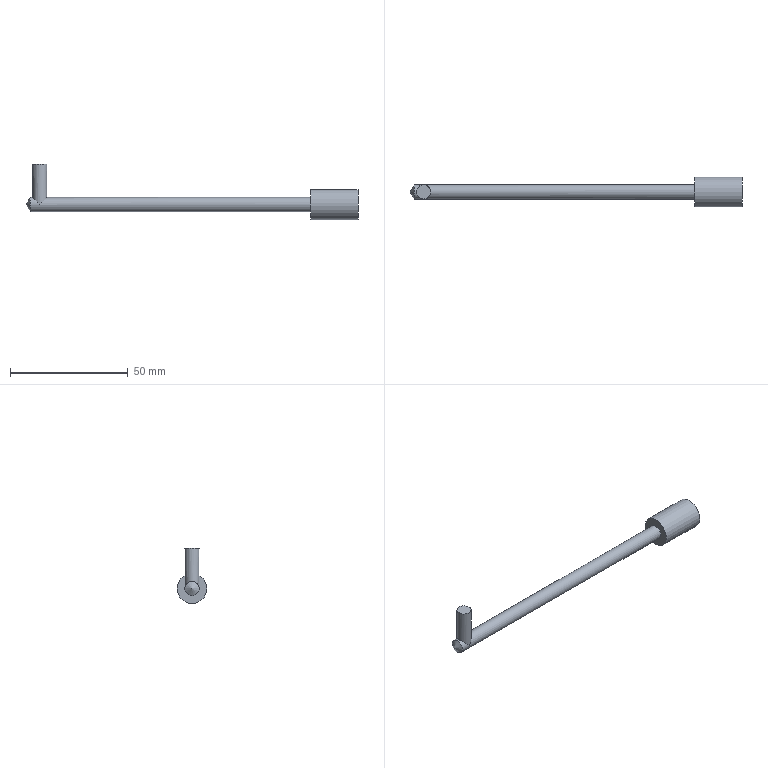Part | NX | features solid 2 | 1 solid | 7 faces | box 140.803 x 12.7 x 23.35 mm | volume 6324 mm3 | plane 3 | cylinder 3 | cone 1 | commonest cylinder face diameters 6 x2 12.7 x1
STEP:
#1=CARTESIAN_POINT('',(155.,30.,-84.));
#2=VERTEX_POINT('',#1);
#3=CARTESIAN_POINT('',(155.,30.,-87.));
#4=DIRECTION('',(-1.,0.,0.));
#5=DIRECTION('',(0.,0.,1.));
#6=AXIS2_PLACEMENT_3D('',#3,#4,#5);
#7=CIRCLE('',#6,3.);
#8=EDGE_CURVE('',#2,#2,#7,.T.);
#9=ORIENTED_EDGE('',*,*,#8,.F.);
#10=EDGE_LOOP('',(#9));
#11=FACE_BOUND('',#10,.T.);
#12=CARTESIAN_POINT('',(155.,30.,-80.65));
#13=VERTEX_POINT('',#12);
#14=CARTESIAN_POINT('',(155.,30.,-87.));
#15=DIRECTION('',(1.,0.,0.));
#16=DIRECTION('',(0.,0.,1.));
#17=AXIS2_PLACEMENT_3D('',#14,#15,#16);
#18=CIRCLE('',#17,6.35);
#19=EDGE_CURVE('',#13,#13,#18,.T.);
#20=ORIENTED_EDGE('',*,*,#19,.F.);
#21=EDGE_LOOP('',(#20));
#22=FACE_BOUND('',#21,.T.);
#23=CARTESIAN_POINT('',(155.,30.,-87.));
#24=DIRECTION('',(-1.,0.,0.));
#25=DIRECTION('',(0.,0.,1.));
#26=AXIS2_PLACEMENT_3D('',#23,#24,#25);
#27=PLANE('',#26);
#28=ADVANCED_FACE('',(#11,#22),#27,.T.);
#29=CARTESIAN_POINT('',(175.,30.,-80.65));
#30=VERTEX_POINT('',#29);
#31=CARTESIAN_POINT('',(175.,30.,-87.));
#32=DIRECTION('',(-1.,0.,0.));
#33=DIRECTION('',(0.,0.,1.));
#34=AXIS2_PLACEMENT_3D('',#31,#32,#33);
#35=CIRCLE('',#34,6.35);
#36=EDGE_CURVE('',#30,#30,#35,.T.);
#37=ORIENTED_EDGE('',*,*,#36,.F.);
#38=EDGE_LOOP('',(#37));
#39=FACE_BOUND('',#38,.T.);
#40=CARTESIAN_POINT('',(175.,30.,-87.));
#41=DIRECTION('',(1.,0.,0.));
#42=DIRECTION('',(0.,0.,-1.));
#43=AXIS2_PLACEMENT_3D('',#40,#41,#42);
#44=PLANE('',#43);
#45=ADVANCED_FACE('',(#39),#44,.T.);
#46=ORIENTED_EDGE('',*,*,#19,.T.);
#47=EDGE_LOOP('',(#46));
#48=FACE_BOUND('',#47,.T.);
#49=ORIENTED_EDGE('',*,*,#36,.T.);
#50=EDGE_LOOP('',(#49));
#51=FACE_BOUND('',#50,.T.);
#52=CARTESIAN_POINT('',(175.,30.,-87.));
#53=DIRECTION('',(-1.,0.,0.));
#54=DIRECTION('',(0.,0.,1.));
#55=AXIS2_PLACEMENT_3D('',#52,#53,#54);
#56=CYLINDRICAL_SURFACE('',#55,6.35);
#57=ADVANCED_FACE('',(#48,#51),#56,.T.);
#58=CARTESIAN_POINT('',(40.,33.,-87.));
#59=VERTEX_POINT('',#58);
#60=CARTESIAN_POINT('',(40.,27.,-87.));
#61=VERTEX_POINT('',#60);
#62=CARTESIAN_POINT('',(40.,30.,-87.));
#63=DIRECTION('',(-0.7071,0.,-0.7071));
#64=DIRECTION('',(-0.7071,0.,0.7071));
#65=AXIS2_PLACEMENT_3D('',#62,#63,#64);
#66=ELLIPSE('',#65,4.243,3.);
#67=EDGE_CURVE('',#59,#61,#66,.F.);
#68=ORIENTED_EDGE('',*,*,#67,.F.);
#69=CARTESIAN_POINT('',(40.,30.,-87.));
#70=DIRECTION('',(-0.7071,0.,0.7071));
#71=DIRECTION('',(-0.7071,0.,-0.7071));
#72=AXIS2_PLACEMENT_3D('',#69,#70,#71);
#73=ELLIPSE('',#72,4.243,3.);
#74=EDGE_CURVE('',#61,#59,#73,.T.);
#75=ORIENTED_EDGE('',*,*,#74,.F.);
#76=EDGE_LOOP('',(#68,#75));
#77=FACE_BOUND('',#76,.T.);
#78=ORIENTED_EDGE('',*,*,#8,.T.);
#79=EDGE_LOOP('',(#78));
#80=FACE_BOUND('',#79,.T.);
#81=CARTESIAN_POINT('',(36.,30.,-84.));
#82=VERTEX_POINT('',#81);
#83=CARTESIAN_POINT('',(36.,30.,-87.));
#84=DIRECTION('',(-1.,0.,0.));
#85=DIRECTION('',(0.,0.,1.));
#86=AXIS2_PLACEMENT_3D('',#83,#84,#85);
#87=CIRCLE('',#86,3.);
#88=EDGE_CURVE('',#82,#82,#87,.T.);
#89=ORIENTED_EDGE('',*,*,#88,.F.);
#90=EDGE_LOOP('',(#89));
#91=FACE_BOUND('',#90,.T.);
#92=CARTESIAN_POINT('',(175.,30.,-87.));
#93=DIRECTION('',(-1.,0.,0.));
#94=DIRECTION('',(0.,0.,1.));
#95=AXIS2_PLACEMENT_3D('',#92,#93,#94);
#96=CYLINDRICAL_SURFACE('',#95,3.);
#97=ADVANCED_FACE('',(#77,#80,#91),#96,.T.);
#98=ORIENTED_EDGE('',*,*,#88,.T.);
#99=EDGE_LOOP('',(#98));
#100=FACE_BOUND('',#99,.T.);
#101=CARTESIAN_POINT('',(34.197,30.,-87.));
#102=VERTEX_POINT('',#101);
#103=VERTEX_LOOP('',#102);
#104=FACE_BOUND('',#103,.T.);
#105=CARTESIAN_POINT('',(34.197,30.,-87.));
#106=DIRECTION('',(1.,0.,0.));
#107=DIRECTION('',(0.,0.,1.));
#108=AXIS2_PLACEMENT_3D('',#105,#106,#107);
#109=CONICAL_SURFACE('',#108,0.,1.03);
#110=ADVANCED_FACE('',(#100,#104),#109,.T.);
#111=CARTESIAN_POINT('',(43.,30.,-70.));
#112=VERTEX_POINT('',#111);
#113=CARTESIAN_POINT('',(40.,30.,-70.));
#114=DIRECTION('',(0.,0.,-1.));
#115=DIRECTION('',(1.,0.,0.));
#116=AXIS2_PLACEMENT_3D('',#113,#114,#115);
#117=CIRCLE('',#116,3.);
#118=EDGE_CURVE('',#112,#112,#117,.T.);
#119=ORIENTED_EDGE('',*,*,#118,.F.);
#120=EDGE_LOOP('',(#119));
#121=FACE_BOUND('',#120,.T.);
#122=CARTESIAN_POINT('',(40.,30.,-70.));
#123=DIRECTION('',(0.,0.,1.));
#124=DIRECTION('',(1.,0.,0.));
#125=AXIS2_PLACEMENT_3D('',#122,#123,#124);
#126=PLANE('',#125);
#127=ADVANCED_FACE('',(#121),#126,.T.);
#128=ORIENTED_EDGE('',*,*,#74,.T.);
#129=ORIENTED_EDGE('',*,*,#67,.T.);
#130=EDGE_LOOP('',(#128,#129));
#131=FACE_BOUND('',#130,.T.);
#132=ORIENTED_EDGE('',*,*,#118,.T.);
#133=EDGE_LOOP('',(#132));
#134=FACE_BOUND('',#133,.T.);
#135=CARTESIAN_POINT('',(40.,30.,-70.));
#136=DIRECTION('',(0.,0.,-1.));
#137=DIRECTION('',(1.,0.,0.));
#138=AXIS2_PLACEMENT_3D('',#135,#136,#137);
#139=CYLINDRICAL_SURFACE('',#138,3.);
#140=ADVANCED_FACE('',(#131,#134),#139,.T.);
#141=CLOSED_SHELL('',(#28,#45,#57,#97,#110,#127,#140));
#142=MANIFOLD_SOLID_BREP('',#141);
#143=(LENGTH_UNIT()NAMED_UNIT(*)SI_UNIT(.MILLI.,.METRE.));
#144=UNCERTAINTY_MEASURE_WITH_UNIT(LENGTH_MEASURE(0.00001),#143,'','');
#145=(NAMED_UNIT(*)PLANE_ANGLE_UNIT()SI_UNIT($,.RADIAN.));
#146=(NAMED_UNIT(*)SI_UNIT($,.STERADIAN.)SOLID_ANGLE_UNIT());
#147=(GEOMETRIC_REPRESENTATION_CONTEXT(3)GLOBAL_UNCERTAINTY_ASSIGNED_CONTEXT((#144))GLOBAL_UNIT_ASSIGNED_CONTEXT((#143,#145,#146))REPRESENTATION_CONTEXT('',''));
#148=ADVANCED_BREP_SHAPE_REPRESENTATION('',(#142),#147);